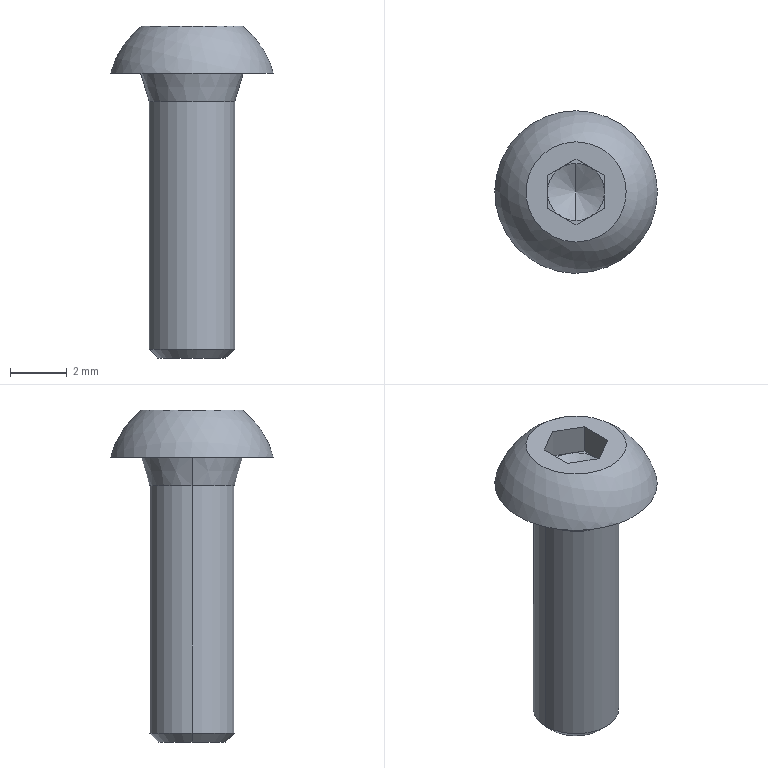Part | SolidWorks | features BaseBody 1 | 1 solid | 24 faces | box 5.7 x 5.7 x 11.65 mm | volume 98.987 mm3 | plane 15 | cone 6 | cylinder 2 | sphere 1 | commonest cylinder face diameters 3 x2
STEP:
#1=CARTESIAN_POINT('',(1.5,0.,-8.694));
#2=VERTEX_POINT('',#1);
#3=CARTESIAN_POINT('',(-1.5,0.,-8.694));
#4=VERTEX_POINT('',#3);
#5=CARTESIAN_POINT('',(0.,0.,-8.694));
#6=DIRECTION('',(0.,0.,1.));
#7=DIRECTION('',(1.,0.,0.));
#8=AXIS2_PLACEMENT_3D('',#5,#6,#7);
#9=CIRCLE('',#8,1.5);
#10=EDGE_CURVE('',#2,#4,#9,.T.);
#11=ORIENTED_EDGE('',*,*,#10,.T.);
#12=CARTESIAN_POINT('',(-1.5,0.,0.));
#13=VERTEX_POINT('',#12);
#14=CARTESIAN_POINT('',(-1.5,0.,-9.));
#15=DIRECTION('',(0.,0.,1.));
#16=VECTOR('',#15,1000.);
#17=LINE('',#14,#16);
#18=EDGE_CURVE('',#4,#13,#17,.T.);
#19=ORIENTED_EDGE('',*,*,#18,.T.);
#20=CARTESIAN_POINT('',(1.5,0.,0.));
#21=VERTEX_POINT('',#20);
#22=CARTESIAN_POINT('',(0.,0.,0.));
#23=DIRECTION('',(0.,0.,-1.));
#24=DIRECTION('',(1.,0.,0.));
#25=AXIS2_PLACEMENT_3D('',#22,#23,#24);
#26=CIRCLE('',#25,1.5);
#27=EDGE_CURVE('',#13,#21,#26,.T.);
#28=ORIENTED_EDGE('',*,*,#27,.T.);
#29=CARTESIAN_POINT('',(1.5,0.,-9.));
#30=DIRECTION('',(0.,0.,1.));
#31=VECTOR('',#30,1000.);
#32=LINE('',#29,#31);
#33=EDGE_CURVE('',#2,#21,#32,.T.);
#34=ORIENTED_EDGE('',*,*,#33,.F.);
#35=EDGE_LOOP('',(#11,#19,#28,#34));
#36=FACE_OUTER_BOUND('',#35,.T.);
#37=CARTESIAN_POINT('',(0.,0.,-9.));
#38=DIRECTION('',(0.,0.,1.));
#39=DIRECTION('',(1.,0.,0.));
#40=AXIS2_PLACEMENT_3D('',#37,#38,#39);
#41=CYLINDRICAL_SURFACE('',#40,1.5);
#42=ADVANCED_FACE('',(#36),#41,.T.);
#43=ORIENTED_EDGE('',*,*,#27,.F.);
#44=CARTESIAN_POINT('',(-1.8,0.,1.));
#45=VERTEX_POINT('',#44);
#46=CARTESIAN_POINT('',(-1.8,0.,1.));
#47=DIRECTION('',(-0.2873,0.,0.9578));
#48=VECTOR('',#47,1000.);
#49=LINE('',#46,#48);
#50=EDGE_CURVE('',#13,#45,#49,.T.);
#51=ORIENTED_EDGE('',*,*,#50,.T.);
#52=CARTESIAN_POINT('',(1.8,0.,1.));
#53=VERTEX_POINT('',#52);
#54=CARTESIAN_POINT('',(0.,0.,1.));
#55=DIRECTION('',(0.,0.,-1.));
#56=DIRECTION('',(1.,0.,0.));
#57=AXIS2_PLACEMENT_3D('',#54,#55,#56);
#58=CIRCLE('',#57,1.8);
#59=EDGE_CURVE('',#45,#53,#58,.T.);
#60=ORIENTED_EDGE('',*,*,#59,.T.);
#61=CARTESIAN_POINT('',(1.8,0.,1.));
#62=DIRECTION('',(0.2873,0.,0.9578));
#63=VECTOR('',#62,1000.);
#64=LINE('',#61,#63);
#65=EDGE_CURVE('',#21,#53,#64,.T.);
#66=ORIENTED_EDGE('',*,*,#65,.F.);
#67=EDGE_LOOP('',(#43,#51,#60,#66));
#68=FACE_OUTER_BOUND('',#67,.T.);
#69=CARTESIAN_POINT('',(0.,0.,1.));
#70=DIRECTION('',(0.,0.,1.));
#71=DIRECTION('',(1.,0.,0.));
#72=AXIS2_PLACEMENT_3D('',#69,#70,#71);
#73=CONICAL_SURFACE('',#72,1.8,0.2915);
#74=ADVANCED_FACE('',(#68),#73,.T.);
#75=CARTESIAN_POINT('',(1.194,0.,-9.));
#76=VERTEX_POINT('',#75);
#77=CARTESIAN_POINT('',(-1.194,0.,-9.));
#78=VERTEX_POINT('',#77);
#79=CARTESIAN_POINT('',(0.,0.,-9.));
#80=DIRECTION('',(0.,0.,1.));
#81=DIRECTION('',(1.,0.,0.));
#82=AXIS2_PLACEMENT_3D('',#79,#80,#81);
#83=CIRCLE('',#82,1.194);
#84=EDGE_CURVE('',#76,#78,#83,.T.);
#85=ORIENTED_EDGE('',*,*,#84,.T.);
#86=CARTESIAN_POINT('',(-1.5,0.,-8.694));
#87=DIRECTION('',(-0.7071,0.,0.7071));
#88=VECTOR('',#87,1000.);
#89=LINE('',#86,#88);
#90=EDGE_CURVE('',#78,#4,#89,.T.);
#91=ORIENTED_EDGE('',*,*,#90,.T.);
#92=ORIENTED_EDGE('',*,*,#10,.F.);
#93=CARTESIAN_POINT('',(1.5,0.,-8.694));
#94=DIRECTION('',(0.7071,0.,0.7071));
#95=VECTOR('',#94,1000.);
#96=LINE('',#93,#95);
#97=EDGE_CURVE('',#76,#2,#96,.T.);
#98=ORIENTED_EDGE('',*,*,#97,.F.);
#99=EDGE_LOOP('',(#85,#91,#92,#98));
#100=FACE_OUTER_BOUND('',#99,.T.);
#101=CARTESIAN_POINT('',(0.,0.,-8.694));
#102=DIRECTION('',(0.,0.,1.));
#103=DIRECTION('',(1.,0.,0.));
#104=AXIS2_PLACEMENT_3D('',#101,#102,#103);
#105=CONICAL_SURFACE('',#104,1.5,0.7854);
#106=ADVANCED_FACE('',(#100),#105,.T.);
#107=CARTESIAN_POINT('',(0.,0.,1.033));
#108=VERTEX_POINT('',#107);
#109=CARTESIAN_POINT('',(0.,-1.,1.61));
#110=VERTEX_POINT('',#109);
#111=CARTESIAN_POINT('',(0.,-1.,1.61));
#112=DIRECTION('',(0.,-0.866,0.5));
#113=VECTOR('',#112,1000.);
#114=LINE('',#111,#113);
#115=EDGE_CURVE('',#108,#110,#114,.T.);
#116=ORIENTED_EDGE('',*,*,#115,.F.);
#117=CARTESIAN_POINT('',(0.,1.,1.61));
#118=VERTEX_POINT('',#117);
#119=CARTESIAN_POINT('',(0.,1.,1.61));
#120=DIRECTION('',(0.,0.866,0.5));
#121=VECTOR('',#120,1000.);
#122=LINE('',#119,#121);
#123=EDGE_CURVE('',#108,#118,#122,.T.);
#124=ORIENTED_EDGE('',*,*,#123,.T.);
#125=CARTESIAN_POINT('',(-0.5,0.866,1.61));
#126=VERTEX_POINT('',#125);
#127=CARTESIAN_POINT('',(0.,0.,1.61));
#128=DIRECTION('',(0.,0.,-1.));
#129=DIRECTION('',(0.,-1.,0.));
#130=AXIS2_PLACEMENT_3D('',#127,#128,#129);
#131=CIRCLE('',#130,1.);
#132=EDGE_CURVE('',#126,#118,#131,.T.);
#133=ORIENTED_EDGE('',*,*,#132,.F.);
#134=CARTESIAN_POINT('',(-1.,0.,1.61));
#135=VERTEX_POINT('',#134);
#136=CARTESIAN_POINT('',(0.,0.,1.61));
#137=DIRECTION('',(0.,0.,-1.));
#138=DIRECTION('',(0.,-1.,0.));
#139=AXIS2_PLACEMENT_3D('',#136,#137,#138);
#140=CIRCLE('',#139,1.);
#141=EDGE_CURVE('',#135,#126,#140,.T.);
#142=ORIENTED_EDGE('',*,*,#141,.F.);
#143=CARTESIAN_POINT('',(-0.5,-0.866,1.61));
#144=VERTEX_POINT('',#143);
#145=CARTESIAN_POINT('',(0.,0.,1.61));
#146=DIRECTION('',(0.,0.,-1.));
#147=DIRECTION('',(0.,-1.,0.));
#148=AXIS2_PLACEMENT_3D('',#145,#146,#147);
#149=CIRCLE('',#148,1.);
#150=EDGE_CURVE('',#144,#135,#149,.T.);
#151=ORIENTED_EDGE('',*,*,#150,.F.);
#152=CARTESIAN_POINT('',(0.,0.,1.61));
#153=DIRECTION('',(0.,0.,-1.));
#154=DIRECTION('',(0.,-1.,0.));
#155=AXIS2_PLACEMENT_3D('',#152,#153,#154);
#156=CIRCLE('',#155,1.);
#157=EDGE_CURVE('',#110,#144,#156,.T.);
#158=ORIENTED_EDGE('',*,*,#157,.F.);
#159=EDGE_LOOP('',(#116,#124,#133,#142,#151,#158));
#160=FACE_OUTER_BOUND('',#159,.T.);
#161=CARTESIAN_POINT('',(0.,0.,1.61));
#162=DIRECTION('',(0.,0.,1.));
#163=DIRECTION('',(0.,-1.,0.));
#164=AXIS2_PLACEMENT_3D('',#161,#162,#163);
#165=CONICAL_SURFACE('',#164,1.,1.047);
#166=ADVANCED_FACE('',(#160),#165,.F.);
#167=ORIENTED_EDGE('',*,*,#18,.F.);
#168=CARTESIAN_POINT('',(0.,0.,-8.694));
#169=DIRECTION('',(0.,0.,1.));
#170=DIRECTION('',(1.,0.,0.));
#171=AXIS2_PLACEMENT_3D('',#168,#169,#170);
#172=CIRCLE('',#171,1.5);
#173=EDGE_CURVE('',#4,#2,#172,.T.);
#174=ORIENTED_EDGE('',*,*,#173,.T.);
#175=ORIENTED_EDGE('',*,*,#33,.T.);
#176=CARTESIAN_POINT('',(0.,0.,0.));
#177=DIRECTION('',(0.,0.,-1.));
#178=DIRECTION('',(1.,0.,0.));
#179=AXIS2_PLACEMENT_3D('',#176,#177,#178);
#180=CIRCLE('',#179,1.5);
#181=EDGE_CURVE('',#21,#13,#180,.T.);
#182=ORIENTED_EDGE('',*,*,#181,.T.);
#183=EDGE_LOOP('',(#167,#174,#175,#182));
#184=FACE_OUTER_BOUND('',#183,.T.);
#185=CARTESIAN_POINT('',(0.,0.,-9.));
#186=DIRECTION('',(0.,0.,1.));
#187=DIRECTION('',(1.,0.,0.));
#188=AXIS2_PLACEMENT_3D('',#185,#186,#187);
#189=CYLINDRICAL_SURFACE('',#188,1.5);
#190=ADVANCED_FACE('',(#184),#189,.T.);
#191=ORIENTED_EDGE('',*,*,#50,.F.);
#192=ORIENTED_EDGE('',*,*,#181,.F.);
#193=ORIENTED_EDGE('',*,*,#65,.T.);
#194=CARTESIAN_POINT('',(0.,0.,1.));
#195=DIRECTION('',(0.,0.,-1.));
#196=DIRECTION('',(1.,0.,0.));
#197=AXIS2_PLACEMENT_3D('',#194,#195,#196);
#198=CIRCLE('',#197,1.8);
#199=EDGE_CURVE('',#53,#45,#198,.T.);
#200=ORIENTED_EDGE('',*,*,#199,.T.);
#201=EDGE_LOOP('',(#191,#192,#193,#200));
#202=FACE_OUTER_BOUND('',#201,.T.);
#203=CARTESIAN_POINT('',(0.,0.,1.));
#204=DIRECTION('',(0.,0.,1.));
#205=DIRECTION('',(1.,0.,0.));
#206=AXIS2_PLACEMENT_3D('',#203,#204,#205);
#207=CONICAL_SURFACE('',#206,1.8,0.2915);
#208=ADVANCED_FACE('',(#202),#207,.T.);
#209=ORIENTED_EDGE('',*,*,#90,.F.);
#210=CARTESIAN_POINT('',(0.,0.,-9.));
#211=DIRECTION('',(0.,0.,1.));
#212=DIRECTION('',(1.,0.,0.));
#213=AXIS2_PLACEMENT_3D('',#210,#211,#212);
#214=CIRCLE('',#213,1.194);
#215=EDGE_CURVE('',#78,#76,#214,.T.);
#216=ORIENTED_EDGE('',*,*,#215,.T.);
#217=ORIENTED_EDGE('',*,*,#97,.T.);
#218=ORIENTED_EDGE('',*,*,#173,.F.);
#219=EDGE_LOOP('',(#209,#216,#217,#218));
#220=FACE_OUTER_BOUND('',#219,.T.);
#221=CARTESIAN_POINT('',(0.,0.,-8.694));
#222=DIRECTION('',(0.,0.,1.));
#223=DIRECTION('',(1.,0.,0.));
#224=AXIS2_PLACEMENT_3D('',#221,#222,#223);
#225=CONICAL_SURFACE('',#224,1.5,0.7854);
#226=ADVANCED_FACE('',(#220),#225,.T.);
#227=CARTESIAN_POINT('',(0.,-2.85,1.));
#228=VERTEX_POINT('',#227);
#229=CARTESIAN_POINT('',(0.,2.85,1.));
#230=VERTEX_POINT('',#229);
#231=CARTESIAN_POINT('',(0.,0.,1.));
#232=DIRECTION('',(0.,0.,1.));
#233=DIRECTION('',(0.,-1.,0.));
#234=AXIS2_PLACEMENT_3D('',#231,#232,#233);
#235=CIRCLE('',#234,2.85);
#236=EDGE_CURVE('',#228,#230,#235,.T.);
#237=ORIENTED_EDGE('',*,*,#236,.F.);
#238=CARTESIAN_POINT('',(0.,0.,1.));
#239=DIRECTION('',(0.,0.,1.));
#240=DIRECTION('',(0.,-1.,0.));
#241=AXIS2_PLACEMENT_3D('',#238,#239,#240);
#242=CIRCLE('',#241,2.85);
#243=EDGE_CURVE('',#230,#228,#242,.T.);
#244=ORIENTED_EDGE('',*,*,#243,.F.);
#245=EDGE_LOOP('',(#237,#244));
#246=FACE_OUTER_BOUND('',#245,.T.);
#247=ORIENTED_EDGE('',*,*,#199,.F.);
#248=ORIENTED_EDGE('',*,*,#59,.F.);
#249=EDGE_LOOP('',(#247,#248));
#250=FACE_BOUND('',#249,.T.);
#251=CARTESIAN_POINT('',(0.,2.85,1.));
#252=DIRECTION('',(0.,0.,1.));
#253=DIRECTION('',(0.,-1.,0.));
#254=AXIS2_PLACEMENT_3D('',#251,#252,#253);
#255=PLANE('',#254);
#256=ADVANCED_FACE('',(#246,#250),#255,.F.);
#257=ORIENTED_EDGE('',*,*,#84,.F.);
#258=ORIENTED_EDGE('',*,*,#215,.F.);
#259=EDGE_LOOP('',(#257,#258));
#260=FACE_OUTER_BOUND('',#259,.T.);
#261=CARTESIAN_POINT('',(1.5,0.,-9.));
#262=DIRECTION('',(0.,0.,-1.));
#263=DIRECTION('',(-1.,0.,0.));
#264=AXIS2_PLACEMENT_3D('',#261,#262,#263);
#265=PLANE('',#264);
#266=ADVANCED_FACE('',(#260),#265,.T.);
#267=CARTESIAN_POINT('',(0.,1.758,2.65));
#268=VERTEX_POINT('',#267);
#269=CARTESIAN_POINT('',(0.,-1.758,2.65));
#270=VERTEX_POINT('',#269);
#271=CARTESIAN_POINT('',(0.,0.,2.65));
#272=DIRECTION('',(0.,0.,-1.));
#273=DIRECTION('',(0.,1.,0.));
#274=AXIS2_PLACEMENT_3D('',#271,#272,#273);
#275=CIRCLE('',#274,1.758);
#276=EDGE_CURVE('',#268,#270,#275,.T.);
#277=ORIENTED_EDGE('',*,*,#276,.T.);
#278=CARTESIAN_POINT('',(0.,0.,2.65));
#279=DIRECTION('',(0.,0.,-1.));
#280=DIRECTION('',(0.,1.,0.));
#281=AXIS2_PLACEMENT_3D('',#278,#279,#280);
#282=CIRCLE('',#281,1.758);
#283=EDGE_CURVE('',#270,#268,#282,.T.);
#284=ORIENTED_EDGE('',*,*,#283,.T.);
#285=EDGE_LOOP('',(#277,#284));
#286=FACE_BOUND('',#285,.T.);
#287=ORIENTED_EDGE('',*,*,#236,.T.);
#288=ORIENTED_EDGE('',*,*,#243,.T.);
#289=EDGE_LOOP('',(#287,#288));
#290=FACE_OUTER_BOUND('',#289,.T.);
#291=CARTESIAN_POINT('',(0.,0.,0.3));
#292=DIRECTION('',(0.2227,0.,0.9749));
#293=DIRECTION('',(-0.9749,0.,0.2227));
#294=AXIS2_PLACEMENT_3D('',#291,#292,#293);
#295=SPHERICAL_SURFACE('',#294,2.935);
#296=ADVANCED_FACE('',(#286,#290),#295,.T.);
#297=ORIENTED_EDGE('',*,*,#276,.F.);
#298=ORIENTED_EDGE('',*,*,#283,.F.);
#299=EDGE_LOOP('',(#297,#298));
#300=FACE_OUTER_BOUND('',#299,.T.);
#301=CARTESIAN_POINT('',(0.,-1.155,2.65));
#302=VERTEX_POINT('',#301);
#303=CARTESIAN_POINT('',(1.,-0.5774,2.65));
#304=VERTEX_POINT('',#303);
#305=CARTESIAN_POINT('',(0.,-1.155,2.65));
#306=DIRECTION('',(0.866,0.5,0.));
#307=VECTOR('',#306,1000.);
#308=LINE('',#305,#307);
#309=EDGE_CURVE('',#302,#304,#308,.T.);
#310=ORIENTED_EDGE('',*,*,#309,.F.);
#311=CARTESIAN_POINT('',(-1.,-0.5774,2.65));
#312=VERTEX_POINT('',#311);
#313=CARTESIAN_POINT('',(-1.,-0.5774,2.65));
#314=DIRECTION('',(0.866,-0.5,0.));
#315=VECTOR('',#314,1000.);
#316=LINE('',#313,#315);
#317=EDGE_CURVE('',#312,#302,#316,.T.);
#318=ORIENTED_EDGE('',*,*,#317,.F.);
#319=CARTESIAN_POINT('',(-1.,0.5774,2.65));
#320=VERTEX_POINT('',#319);
#321=CARTESIAN_POINT('',(-1.,0.,2.65));
#322=DIRECTION('',(0.,-1.,0.));
#323=VECTOR('',#322,1000.);
#324=LINE('',#321,#323);
#325=EDGE_CURVE('',#320,#312,#324,.T.);
#326=ORIENTED_EDGE('',*,*,#325,.F.);
#327=CARTESIAN_POINT('',(0.,1.155,2.65));
#328=VERTEX_POINT('',#327);
#329=CARTESIAN_POINT('',(0.,1.155,2.65));
#330=DIRECTION('',(-0.866,-0.5,0.));
#331=VECTOR('',#330,1000.);
#332=LINE('',#329,#331);
#333=EDGE_CURVE('',#328,#320,#332,.T.);
#334=ORIENTED_EDGE('',*,*,#333,.F.);
#335=CARTESIAN_POINT('',(1.,0.5774,2.65));
#336=VERTEX_POINT('',#335);
#337=CARTESIAN_POINT('',(1.,0.5774,2.65));
#338=DIRECTION('',(-0.866,0.5,0.));
#339=VECTOR('',#338,1000.);
#340=LINE('',#337,#339);
#341=EDGE_CURVE('',#336,#328,#340,.T.);
#342=ORIENTED_EDGE('',*,*,#341,.F.);
#343=CARTESIAN_POINT('',(1.,0.,2.65));
#344=DIRECTION('',(0.,1.,0.));
#345=VECTOR('',#344,1000.);
#346=LINE('',#343,#345);
#347=EDGE_CURVE('',#304,#336,#346,.T.);
#348=ORIENTED_EDGE('',*,*,#347,.F.);
#349=EDGE_LOOP('',(#310,#318,#326,#334,#342,#348));
#350=FACE_BOUND('',#349,.T.);
#351=CARTESIAN_POINT('',(0.,0.,2.65));
#352=DIRECTION('',(0.,0.,-1.));
#353=DIRECTION('',(0.,1.,0.));
#354=AXIS2_PLACEMENT_3D('',#351,#352,#353);
#355=PLANE('',#354);
#356=ADVANCED_FACE('',(#300,#350),#355,.F.);
#357=CARTESIAN_POINT('',(1.,0.5774,1.61));
#358=VERTEX_POINT('',#357);
#359=CARTESIAN_POINT('',(1.,0.5774,1.61));
#360=DIRECTION('',(0.,0.,1.));
#361=VECTOR('',#360,1000.);
#362=LINE('',#359,#361);
#363=EDGE_CURVE('',#358,#336,#362,.T.);
#364=ORIENTED_EDGE('',*,*,#363,.F.);
#365=CARTESIAN_POINT('',(1.,0.,1.61));
#366=VERTEX_POINT('',#365);
#367=CARTESIAN_POINT('',(1.,-0.5774,1.61));
#368=DIRECTION('',(0.,1.,0.));
#369=VECTOR('',#368,1000.);
#370=LINE('',#367,#369);
#371=EDGE_CURVE('',#366,#358,#370,.T.);
#372=ORIENTED_EDGE('',*,*,#371,.F.);
#373=CARTESIAN_POINT('',(1.,-0.5774,1.61));
#374=VERTEX_POINT('',#373);
#375=CARTESIAN_POINT('',(1.,-0.5774,1.61));
#376=DIRECTION('',(0.,1.,0.));
#377=VECTOR('',#376,1000.);
#378=LINE('',#375,#377);
#379=EDGE_CURVE('',#374,#366,#378,.T.);
#380=ORIENTED_EDGE('',*,*,#379,.F.);
#381=CARTESIAN_POINT('',(1.,-0.5774,1.61));
#382=DIRECTION('',(0.,0.,-1.));
#383=VECTOR('',#382,1000.);
#384=LINE('',#381,#383);
#385=EDGE_CURVE('',#304,#374,#384,.T.);
#386=ORIENTED_EDGE('',*,*,#385,.F.);
#387=ORIENTED_EDGE('',*,*,#347,.T.);
#388=EDGE_LOOP('',(#364,#372,#380,#386,#387));
#389=FACE_OUTER_BOUND('',#388,.T.);
#390=CARTESIAN_POINT('',(1.,-0.5774,1.61));
#391=DIRECTION('',(1.,0.,0.));
#392=DIRECTION('',(0.,0.,-1.));
#393=AXIS2_PLACEMENT_3D('',#390,#391,#392);
#394=PLANE('',#393);
#395=ADVANCED_FACE('',(#389),#394,.F.);
#396=ORIENTED_EDGE('',*,*,#385,.T.);
#397=CARTESIAN_POINT('',(0.5,-0.866,1.61));
#398=VERTEX_POINT('',#397);
#399=CARTESIAN_POINT('',(0.,-1.155,1.61));
#400=DIRECTION('',(0.866,0.5,0.));
#401=VECTOR('',#400,1000.);
#402=LINE('',#399,#401);
#403=EDGE_CURVE('',#398,#374,#402,.T.);
#404=ORIENTED_EDGE('',*,*,#403,.F.);
#405=CARTESIAN_POINT('',(0.,-1.155,1.61));
#406=VERTEX_POINT('',#405);
#407=CARTESIAN_POINT('',(0.,-1.155,1.61));
#408=DIRECTION('',(0.866,0.5,0.));
#409=VECTOR('',#408,1000.);
#410=LINE('',#407,#409);
#411=EDGE_CURVE('',#406,#398,#410,.T.);
#412=ORIENTED_EDGE('',*,*,#411,.F.);
#413=CARTESIAN_POINT('',(0.,-1.155,1.61));
#414=DIRECTION('',(0.,0.,-1.));
#415=VECTOR('',#414,1000.);
#416=LINE('',#413,#415);
#417=EDGE_CURVE('',#302,#406,#416,.T.);
#418=ORIENTED_EDGE('',*,*,#417,.F.);
#419=ORIENTED_EDGE('',*,*,#309,.T.);
#420=EDGE_LOOP('',(#396,#404,#412,#418,#419));
#421=FACE_OUTER_BOUND('',#420,.T.);
#422=CARTESIAN_POINT('',(0.,-1.155,1.61));
#423=DIRECTION('',(0.5,-0.866,0.));
#424=DIRECTION('',(0.866,0.5,0.));
#425=AXIS2_PLACEMENT_3D('',#422,#423,#424);
#426=PLANE('',#425);
#427=ADVANCED_FACE('',(#421),#426,.F.);
#428=ORIENTED_EDGE('',*,*,#417,.T.);
#429=CARTESIAN_POINT('',(-1.,-0.5774,1.61));
#430=DIRECTION('',(0.866,-0.5,0.));
#431=VECTOR('',#430,1000.);
#432=LINE('',#429,#431);
#433=EDGE_CURVE('',#144,#406,#432,.T.);
#434=ORIENTED_EDGE('',*,*,#433,.F.);
#435=CARTESIAN_POINT('',(-1.,-0.5774,1.61));
#436=VERTEX_POINT('',#435);
#437=CARTESIAN_POINT('',(-1.,-0.5774,1.61));
#438=DIRECTION('',(0.866,-0.5,0.));
#439=VECTOR('',#438,1000.);
#440=LINE('',#437,#439);
#441=EDGE_CURVE('',#436,#144,#440,.T.);
#442=ORIENTED_EDGE('',*,*,#441,.F.);
#443=CARTESIAN_POINT('',(-1.,-0.5774,1.61));
#444=DIRECTION('',(0.,0.,-1.));
#445=VECTOR('',#444,1000.);
#446=LINE('',#443,#445);
#447=EDGE_CURVE('',#312,#436,#446,.T.);
#448=ORIENTED_EDGE('',*,*,#447,.F.);
#449=ORIENTED_EDGE('',*,*,#317,.T.);
#450=EDGE_LOOP('',(#428,#434,#442,#448,#449));
#451=FACE_OUTER_BOUND('',#450,.T.);
#452=CARTESIAN_POINT('',(-1.,-0.5774,1.61));
#453=DIRECTION('',(-0.5,-0.866,0.));
#454=DIRECTION('',(0.866,-0.5,0.));
#455=AXIS2_PLACEMENT_3D('',#452,#453,#454);
#456=PLANE('',#455);
#457=ADVANCED_FACE('',(#451),#456,.F.);
#458=ORIENTED_EDGE('',*,*,#447,.T.);
#459=CARTESIAN_POINT('',(-1.,0.5774,1.61));
#460=DIRECTION('',(0.,-1.,0.));
#461=VECTOR('',#460,1000.);
#462=LINE('',#459,#461);
#463=EDGE_CURVE('',#135,#436,#462,.T.);
#464=ORIENTED_EDGE('',*,*,#463,.F.);
#465=CARTESIAN_POINT('',(-1.,0.5774,1.61));
#466=VERTEX_POINT('',#465);
#467=CARTESIAN_POINT('',(-1.,0.5774,1.61));
#468=DIRECTION('',(0.,-1.,0.));
#469=VECTOR('',#468,1000.);
#470=LINE('',#467,#469);
#471=EDGE_CURVE('',#466,#135,#470,.T.);
#472=ORIENTED_EDGE('',*,*,#471,.F.);
#473=CARTESIAN_POINT('',(-1.,0.5774,1.61));
#474=DIRECTION('',(0.,0.,-1.));
#475=VECTOR('',#474,1000.);
#476=LINE('',#473,#475);
#477=EDGE_CURVE('',#320,#466,#476,.T.);
#478=ORIENTED_EDGE('',*,*,#477,.F.);
#479=ORIENTED_EDGE('',*,*,#325,.T.);
#480=EDGE_LOOP('',(#458,#464,#472,#478,#479));
#481=FACE_OUTER_BOUND('',#480,.T.);
#482=CARTESIAN_POINT('',(-1.,0.5774,1.61));
#483=DIRECTION('',(-1.,0.,0.));
#484=DIRECTION('',(0.,-1.,0.));
#485=AXIS2_PLACEMENT_3D('',#482,#483,#484);
#486=PLANE('',#485);
#487=ADVANCED_FACE('',(#481),#486,.F.);
#488=ORIENTED_EDGE('',*,*,#477,.T.);
#489=CARTESIAN_POINT('',(0.,1.155,1.61));
#490=DIRECTION('',(-0.866,-0.5,0.));
#491=VECTOR('',#490,1000.);
#492=LINE('',#489,#491);
#493=EDGE_CURVE('',#126,#466,#492,.T.);
#494=ORIENTED_EDGE('',*,*,#493,.F.);
#495=CARTESIAN_POINT('',(0.,1.155,1.61));
#496=VERTEX_POINT('',#495);
#497=CARTESIAN_POINT('',(0.,1.155,1.61));
#498=DIRECTION('',(-0.866,-0.5,0.));
#499=VECTOR('',#498,1000.);
#500=LINE('',#497,#499);
#501=EDGE_CURVE('',#496,#126,#500,.T.);
#502=ORIENTED_EDGE('',*,*,#501,.F.);
#503=CARTESIAN_POINT('',(0.,1.155,1.61));
#504=DIRECTION('',(0.,0.,-1.));
#505=VECTOR('',#504,1000.);
#506=LINE('',#503,#505);
#507=EDGE_CURVE('',#328,#496,#506,.T.);
#508=ORIENTED_EDGE('',*,*,#507,.F.);
#509=ORIENTED_EDGE('',*,*,#333,.T.);
#510=EDGE_LOOP('',(#488,#494,#502,#508,#509));
#511=FACE_OUTER_BOUND('',#510,.T.);
#512=CARTESIAN_POINT('',(0.,1.155,1.61));
#513=DIRECTION('',(-0.5,0.866,0.));
#514=DIRECTION('',(-0.866,-0.5,0.));
#515=AXIS2_PLACEMENT_3D('',#512,#513,#514);
#516=PLANE('',#515);
#517=ADVANCED_FACE('',(#511),#516,.F.);
#518=ORIENTED_EDGE('',*,*,#507,.T.);
#519=CARTESIAN_POINT('',(0.5,0.866,1.61));
#520=VERTEX_POINT('',#519);
#521=CARTESIAN_POINT('',(1.,0.5774,1.61));
#522=DIRECTION('',(-0.866,0.5,0.));
#523=VECTOR('',#522,1000.);
#524=LINE('',#521,#523);
#525=EDGE_CURVE('',#520,#496,#524,.T.);
#526=ORIENTED_EDGE('',*,*,#525,.F.);
#527=CARTESIAN_POINT('',(1.,0.5774,1.61));
#528=DIRECTION('',(-0.866,0.5,0.));
#529=VECTOR('',#528,1000.);
#530=LINE('',#527,#529);
#531=EDGE_CURVE('',#358,#520,#530,.T.);
#532=ORIENTED_EDGE('',*,*,#531,.F.);
#533=ORIENTED_EDGE('',*,*,#363,.T.);
#534=ORIENTED_EDGE('',*,*,#341,.T.);
#535=EDGE_LOOP('',(#518,#526,#532,#533,#534));
#536=FACE_OUTER_BOUND('',#535,.T.);
#537=CARTESIAN_POINT('',(1.,0.5774,1.61));
#538=DIRECTION('',(0.5,0.866,0.));
#539=DIRECTION('',(-0.866,0.5,0.));
#540=AXIS2_PLACEMENT_3D('',#537,#538,#539);
#541=PLANE('',#540);
#542=ADVANCED_FACE('',(#536),#541,.F.);
#543=CARTESIAN_POINT('',(0.,0.,1.61));
#544=DIRECTION('',(0.,0.,-1.));
#545=DIRECTION('',(0.,-1.,0.));
#546=AXIS2_PLACEMENT_3D('',#543,#544,#545);
#547=CIRCLE('',#546,1.);
#548=EDGE_CURVE('',#520,#366,#547,.T.);
#549=ORIENTED_EDGE('',*,*,#548,.T.);
#550=ORIENTED_EDGE('',*,*,#371,.T.);
#551=ORIENTED_EDGE('',*,*,#531,.T.);
#552=EDGE_LOOP('',(#549,#550,#551));
#553=FACE_OUTER_BOUND('',#552,.T.);
#554=CARTESIAN_POINT('',(0.,0.,1.61));
#555=DIRECTION('',(0.,0.,1.));
#556=DIRECTION('',(1.,0.,0.));
#557=AXIS2_PLACEMENT_3D('',#554,#555,#556);
#558=PLANE('',#557);
#559=ADVANCED_FACE('',(#553),#558,.T.);
#560=CARTESIAN_POINT('',(0.,0.,1.61));
#561=DIRECTION('',(0.,0.,-1.));
#562=DIRECTION('',(0.,-1.,0.));
#563=AXIS2_PLACEMENT_3D('',#560,#561,#562);
#564=CIRCLE('',#563,1.);
#565=EDGE_CURVE('',#366,#398,#564,.T.);
#566=ORIENTED_EDGE('',*,*,#565,.T.);
#567=ORIENTED_EDGE('',*,*,#403,.T.);
#568=ORIENTED_EDGE('',*,*,#379,.T.);
#569=EDGE_LOOP('',(#566,#567,#568));
#570=FACE_OUTER_BOUND('',#569,.T.);
#571=CARTESIAN_POINT('',(0.,0.,1.61));
#572=DIRECTION('',(0.,0.,1.));
#573=DIRECTION('',(1.,0.,0.));
#574=AXIS2_PLACEMENT_3D('',#571,#572,#573);
#575=PLANE('',#574);
#576=ADVANCED_FACE('',(#570),#575,.T.);
#577=CARTESIAN_POINT('',(0.,0.,1.61));
#578=DIRECTION('',(0.,0.,-1.));
#579=DIRECTION('',(0.,-1.,0.));
#580=AXIS2_PLACEMENT_3D('',#577,#578,#579);
#581=CIRCLE('',#580,1.);
#582=EDGE_CURVE('',#398,#110,#581,.T.);
#583=ORIENTED_EDGE('',*,*,#582,.T.);
#584=ORIENTED_EDGE('',*,*,#157,.T.);
#585=ORIENTED_EDGE('',*,*,#433,.T.);
#586=ORIENTED_EDGE('',*,*,#411,.T.);
#587=EDGE_LOOP('',(#583,#584,#585,#586));
#588=FACE_OUTER_BOUND('',#587,.T.);
#589=CARTESIAN_POINT('',(0.,0.,1.61));
#590=DIRECTION('',(0.,0.,1.));
#591=DIRECTION('',(1.,0.,0.));
#592=AXIS2_PLACEMENT_3D('',#589,#590,#591);
#593=PLANE('',#592);
#594=ADVANCED_FACE('',(#588),#593,.T.);
#595=ORIENTED_EDGE('',*,*,#150,.T.);
#596=ORIENTED_EDGE('',*,*,#463,.T.);
#597=ORIENTED_EDGE('',*,*,#441,.T.);
#598=EDGE_LOOP('',(#595,#596,#597));
#599=FACE_OUTER_BOUND('',#598,.T.);
#600=CARTESIAN_POINT('',(0.,0.,1.61));
#601=DIRECTION('',(0.,0.,1.));
#602=DIRECTION('',(1.,0.,0.));
#603=AXIS2_PLACEMENT_3D('',#600,#601,#602);
#604=PLANE('',#603);
#605=ADVANCED_FACE('',(#599),#604,.T.);
#606=ORIENTED_EDGE('',*,*,#141,.T.);
#607=ORIENTED_EDGE('',*,*,#493,.T.);
#608=ORIENTED_EDGE('',*,*,#471,.T.);
#609=EDGE_LOOP('',(#606,#607,#608));
#610=FACE_OUTER_BOUND('',#609,.T.);
#611=CARTESIAN_POINT('',(0.,0.,1.61));
#612=DIRECTION('',(0.,0.,1.));
#613=DIRECTION('',(1.,0.,0.));
#614=AXIS2_PLACEMENT_3D('',#611,#612,#613);
#615=PLANE('',#614);
#616=ADVANCED_FACE('',(#610),#615,.T.);
#617=ORIENTED_EDGE('',*,*,#132,.T.);
#618=CARTESIAN_POINT('',(0.,0.,1.61));
#619=DIRECTION('',(0.,0.,-1.));
#620=DIRECTION('',(0.,-1.,0.));
#621=AXIS2_PLACEMENT_3D('',#618,#619,#620);
#622=CIRCLE('',#621,1.);
#623=EDGE_CURVE('',#118,#520,#622,.T.);
#624=ORIENTED_EDGE('',*,*,#623,.T.);
#625=ORIENTED_EDGE('',*,*,#525,.T.);
#626=ORIENTED_EDGE('',*,*,#501,.T.);
#627=EDGE_LOOP('',(#617,#624,#625,#626));
#628=FACE_OUTER_BOUND('',#627,.T.);
#629=CARTESIAN_POINT('',(0.,0.,1.61));
#630=DIRECTION('',(0.,0.,1.));
#631=DIRECTION('',(1.,0.,0.));
#632=AXIS2_PLACEMENT_3D('',#629,#630,#631);
#633=PLANE('',#632);
#634=ADVANCED_FACE('',(#628),#633,.T.);
#635=ORIENTED_EDGE('',*,*,#123,.F.);
#636=ORIENTED_EDGE('',*,*,#115,.T.);
#637=ORIENTED_EDGE('',*,*,#582,.F.);
#638=ORIENTED_EDGE('',*,*,#565,.F.);
#639=ORIENTED_EDGE('',*,*,#548,.F.);
#640=ORIENTED_EDGE('',*,*,#623,.F.);
#641=EDGE_LOOP('',(#635,#636,#637,#638,#639,#640));
#642=FACE_OUTER_BOUND('',#641,.T.);
#643=CARTESIAN_POINT('',(0.,0.,1.61));
#644=DIRECTION('',(0.,0.,1.));
#645=DIRECTION('',(0.,-1.,0.));
#646=AXIS2_PLACEMENT_3D('',#643,#644,#645);
#647=CONICAL_SURFACE('',#646,1.,1.047);
#648=ADVANCED_FACE('',(#642),#647,.F.);
#649=CLOSED_SHELL('',(#42,#74,#106,#166,#190,#208,#226,#256,#266,#296,#356,#395,#427,#457,#487,#517,#542,#559,#576,#594,#605,#616,#634,#648));
#650=MANIFOLD_SOLID_BREP('',#649);
#651=CARTESIAN_POINT('',(0.,0.,0.));
#652=DIRECTION('',(0.,0.,1.));
#653=DIRECTION('',(1.,0.,0.));
#654=AXIS2_PLACEMENT_3D('',#651,#652,#653);
#655=(LENGTH_UNIT()NAMED_UNIT(*)SI_UNIT(.MILLI.,.METRE.));
#656=UNCERTAINTY_MEASURE_WITH_UNIT(LENGTH_MEASURE(0.00001),#655,'','');
#657=(NAMED_UNIT(*)PLANE_ANGLE_UNIT()SI_UNIT($,.RADIAN.));
#658=(NAMED_UNIT(*)SI_UNIT($,.STERADIAN.)SOLID_ANGLE_UNIT());
#659=(GEOMETRIC_REPRESENTATION_CONTEXT(3)GLOBAL_UNCERTAINTY_ASSIGNED_CONTEXT((#656))GLOBAL_UNIT_ASSIGNED_CONTEXT((#655,#657,#658))REPRESENTATION_CONTEXT('',''));
#660=ADVANCED_BREP_SHAPE_REPRESENTATION('',(#650,#654),#659);